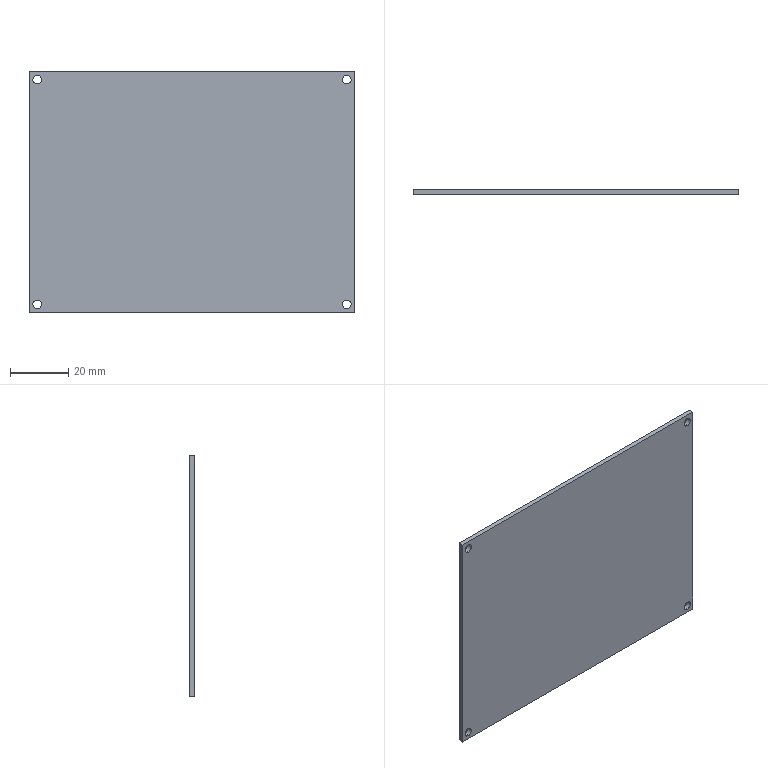Part | SolidWorks | features Extrusion 1 | 1 solid | 14 faces | box 111.5 x 1.75 x 82.6 mm | volume 16068 mm3 | cylinder 8 | plane 6 | commonest cylinder face diameters 3 x8
STEP:
#1=CARTESIAN_POINT('',(-53.,1.75,37.));
#2=VERTEX_POINT('',#1);
#3=CARTESIAN_POINT('',(-53.,1.75,40.));
#4=VERTEX_POINT('',#3);
#5=CARTESIAN_POINT('',(-53.,1.75,38.5));
#6=DIRECTION('',(0.,1.,0.));
#7=DIRECTION('',(0.,0.,-1.));
#8=AXIS2_PLACEMENT_3D('',#5,#6,#7);
#9=CIRCLE('',#8,1.5);
#10=EDGE_CURVE('',#2,#4,#9,.T.);
#11=ORIENTED_EDGE('',*,*,#10,.T.);
#12=CARTESIAN_POINT('',(-53.,0.,40.));
#13=VERTEX_POINT('',#12);
#14=CARTESIAN_POINT('',(-53.,1.75,40.));
#15=DIRECTION('',(0.,-1.,0.));
#16=VECTOR('',#15,1000.);
#17=LINE('',#14,#16);
#18=EDGE_CURVE('',#4,#13,#17,.T.);
#19=ORIENTED_EDGE('',*,*,#18,.T.);
#20=CARTESIAN_POINT('',(-53.,0.,37.));
#21=VERTEX_POINT('',#20);
#22=CARTESIAN_POINT('',(-53.,0.,38.5));
#23=DIRECTION('',(0.,1.,0.));
#24=DIRECTION('',(0.,0.,-1.));
#25=AXIS2_PLACEMENT_3D('',#22,#23,#24);
#26=CIRCLE('',#25,1.5);
#27=EDGE_CURVE('',#21,#13,#26,.T.);
#28=ORIENTED_EDGE('',*,*,#27,.F.);
#29=CARTESIAN_POINT('',(-53.,1.75,37.));
#30=DIRECTION('',(0.,-1.,0.));
#31=VECTOR('',#30,1000.);
#32=LINE('',#29,#31);
#33=EDGE_CURVE('',#2,#21,#32,.T.);
#34=ORIENTED_EDGE('',*,*,#33,.F.);
#35=EDGE_LOOP('',(#11,#19,#28,#34));
#36=FACE_OUTER_BOUND('',#35,.T.);
#37=CARTESIAN_POINT('',(-53.,1.75,38.5));
#38=DIRECTION('',(0.,-1.,0.));
#39=DIRECTION('',(0.,0.,-1.));
#40=AXIS2_PLACEMENT_3D('',#37,#38,#39);
#41=CYLINDRICAL_SURFACE('',#40,1.5);
#42=ADVANCED_FACE('',(#36),#41,.F.);
#43=CARTESIAN_POINT('',(53.,1.75,37.));
#44=VERTEX_POINT('',#43);
#45=CARTESIAN_POINT('',(53.,1.75,40.));
#46=VERTEX_POINT('',#45);
#47=CARTESIAN_POINT('',(53.,1.75,38.5));
#48=DIRECTION('',(0.,1.,0.));
#49=DIRECTION('',(0.,0.,1.));
#50=AXIS2_PLACEMENT_3D('',#47,#48,#49);
#51=CIRCLE('',#50,1.5);
#52=EDGE_CURVE('',#44,#46,#51,.T.);
#53=ORIENTED_EDGE('',*,*,#52,.T.);
#54=CARTESIAN_POINT('',(53.,0.,40.));
#55=VERTEX_POINT('',#54);
#56=CARTESIAN_POINT('',(53.,1.75,40.));
#57=DIRECTION('',(0.,-1.,0.));
#58=VECTOR('',#57,1000.);
#59=LINE('',#56,#58);
#60=EDGE_CURVE('',#46,#55,#59,.T.);
#61=ORIENTED_EDGE('',*,*,#60,.T.);
#62=CARTESIAN_POINT('',(53.,0.,37.));
#63=VERTEX_POINT('',#62);
#64=CARTESIAN_POINT('',(53.,0.,38.5));
#65=DIRECTION('',(0.,1.,0.));
#66=DIRECTION('',(0.,0.,1.));
#67=AXIS2_PLACEMENT_3D('',#64,#65,#66);
#68=CIRCLE('',#67,1.5);
#69=EDGE_CURVE('',#63,#55,#68,.T.);
#70=ORIENTED_EDGE('',*,*,#69,.F.);
#71=CARTESIAN_POINT('',(53.,1.75,37.));
#72=DIRECTION('',(0.,-1.,0.));
#73=VECTOR('',#72,1000.);
#74=LINE('',#71,#73);
#75=EDGE_CURVE('',#44,#63,#74,.T.);
#76=ORIENTED_EDGE('',*,*,#75,.F.);
#77=EDGE_LOOP('',(#53,#61,#70,#76));
#78=FACE_OUTER_BOUND('',#77,.T.);
#79=CARTESIAN_POINT('',(53.,1.75,38.5));
#80=DIRECTION('',(0.,-1.,0.));
#81=DIRECTION('',(0.,0.,-1.));
#82=AXIS2_PLACEMENT_3D('',#79,#80,#81);
#83=CYLINDRICAL_SURFACE('',#82,1.5);
#84=ADVANCED_FACE('',(#78),#83,.F.);
#85=CARTESIAN_POINT('',(53.,1.75,-40.));
#86=VERTEX_POINT('',#85);
#87=CARTESIAN_POINT('',(53.,1.75,-37.));
#88=VERTEX_POINT('',#87);
#89=CARTESIAN_POINT('',(53.,1.75,-38.5));
#90=DIRECTION('',(0.,1.,0.));
#91=DIRECTION('',(0.,0.,-1.));
#92=AXIS2_PLACEMENT_3D('',#89,#90,#91);
#93=CIRCLE('',#92,1.5);
#94=EDGE_CURVE('',#86,#88,#93,.T.);
#95=ORIENTED_EDGE('',*,*,#94,.T.);
#96=CARTESIAN_POINT('',(53.,0.,-37.));
#97=VERTEX_POINT('',#96);
#98=CARTESIAN_POINT('',(53.,1.75,-37.));
#99=DIRECTION('',(0.,-1.,0.));
#100=VECTOR('',#99,1000.);
#101=LINE('',#98,#100);
#102=EDGE_CURVE('',#88,#97,#101,.T.);
#103=ORIENTED_EDGE('',*,*,#102,.T.);
#104=CARTESIAN_POINT('',(53.,0.,-40.));
#105=VERTEX_POINT('',#104);
#106=CARTESIAN_POINT('',(53.,0.,-38.5));
#107=DIRECTION('',(0.,1.,0.));
#108=DIRECTION('',(0.,0.,-1.));
#109=AXIS2_PLACEMENT_3D('',#106,#107,#108);
#110=CIRCLE('',#109,1.5);
#111=EDGE_CURVE('',#105,#97,#110,.T.);
#112=ORIENTED_EDGE('',*,*,#111,.F.);
#113=CARTESIAN_POINT('',(53.,1.75,-40.));
#114=DIRECTION('',(0.,-1.,0.));
#115=VECTOR('',#114,1000.);
#116=LINE('',#113,#115);
#117=EDGE_CURVE('',#86,#105,#116,.T.);
#118=ORIENTED_EDGE('',*,*,#117,.F.);
#119=EDGE_LOOP('',(#95,#103,#112,#118));
#120=FACE_OUTER_BOUND('',#119,.T.);
#121=CARTESIAN_POINT('',(53.,1.75,-38.5));
#122=DIRECTION('',(0.,-1.,0.));
#123=DIRECTION('',(0.,0.,-1.));
#124=AXIS2_PLACEMENT_3D('',#121,#122,#123);
#125=CYLINDRICAL_SURFACE('',#124,1.5);
#126=ADVANCED_FACE('',(#120),#125,.F.);
#127=CARTESIAN_POINT('',(-53.,1.75,-40.));
#128=VERTEX_POINT('',#127);
#129=CARTESIAN_POINT('',(-53.,1.75,-37.));
#130=VERTEX_POINT('',#129);
#131=CARTESIAN_POINT('',(-53.,1.75,-38.5));
#132=DIRECTION('',(0.,1.,0.));
#133=DIRECTION('',(0.,0.,1.));
#134=AXIS2_PLACEMENT_3D('',#131,#132,#133);
#135=CIRCLE('',#134,1.5);
#136=EDGE_CURVE('',#128,#130,#135,.T.);
#137=ORIENTED_EDGE('',*,*,#136,.T.);
#138=CARTESIAN_POINT('',(-53.,0.,-37.));
#139=VERTEX_POINT('',#138);
#140=CARTESIAN_POINT('',(-53.,1.75,-37.));
#141=DIRECTION('',(0.,-1.,0.));
#142=VECTOR('',#141,1000.);
#143=LINE('',#140,#142);
#144=EDGE_CURVE('',#130,#139,#143,.T.);
#145=ORIENTED_EDGE('',*,*,#144,.T.);
#146=CARTESIAN_POINT('',(-53.,0.,-40.));
#147=VERTEX_POINT('',#146);
#148=CARTESIAN_POINT('',(-53.,0.,-38.5));
#149=DIRECTION('',(0.,1.,0.));
#150=DIRECTION('',(0.,0.,1.));
#151=AXIS2_PLACEMENT_3D('',#148,#149,#150);
#152=CIRCLE('',#151,1.5);
#153=EDGE_CURVE('',#147,#139,#152,.T.);
#154=ORIENTED_EDGE('',*,*,#153,.F.);
#155=CARTESIAN_POINT('',(-53.,1.75,-40.));
#156=DIRECTION('',(0.,-1.,0.));
#157=VECTOR('',#156,1000.);
#158=LINE('',#155,#157);
#159=EDGE_CURVE('',#128,#147,#158,.T.);
#160=ORIENTED_EDGE('',*,*,#159,.F.);
#161=EDGE_LOOP('',(#137,#145,#154,#160));
#162=FACE_OUTER_BOUND('',#161,.T.);
#163=CARTESIAN_POINT('',(-53.,1.75,-38.5));
#164=DIRECTION('',(0.,-1.,0.));
#165=DIRECTION('',(0.,0.,-1.));
#166=AXIS2_PLACEMENT_3D('',#163,#164,#165);
#167=CYLINDRICAL_SURFACE('',#166,1.5);
#168=ADVANCED_FACE('',(#162),#167,.F.);
#169=ORIENTED_EDGE('',*,*,#52,.F.);
#170=CARTESIAN_POINT('',(53.,1.75,38.5));
#171=DIRECTION('',(0.,1.,0.));
#172=DIRECTION('',(0.,0.,1.));
#173=AXIS2_PLACEMENT_3D('',#170,#171,#172);
#174=CIRCLE('',#173,1.5);
#175=EDGE_CURVE('',#46,#44,#174,.T.);
#176=ORIENTED_EDGE('',*,*,#175,.F.);
#177=EDGE_LOOP('',(#169,#176));
#178=FACE_BOUND('',#177,.T.);
#179=ORIENTED_EDGE('',*,*,#136,.F.);
#180=CARTESIAN_POINT('',(-53.,1.75,-38.5));
#181=DIRECTION('',(0.,1.,0.));
#182=DIRECTION('',(0.,0.,1.));
#183=AXIS2_PLACEMENT_3D('',#180,#181,#182);
#184=CIRCLE('',#183,1.5);
#185=EDGE_CURVE('',#130,#128,#184,.T.);
#186=ORIENTED_EDGE('',*,*,#185,.F.);
#187=EDGE_LOOP('',(#179,#186));
#188=FACE_BOUND('',#187,.T.);
#189=CARTESIAN_POINT('',(55.75,1.75,41.3));
#190=VERTEX_POINT('',#189);
#191=CARTESIAN_POINT('',(55.75,1.75,-41.3));
#192=VERTEX_POINT('',#191);
#193=CARTESIAN_POINT('',(55.75,1.75,41.3));
#194=DIRECTION('',(0.,0.,-1.));
#195=VECTOR('',#194,1000.);
#196=LINE('',#193,#195);
#197=EDGE_CURVE('',#190,#192,#196,.T.);
#198=ORIENTED_EDGE('',*,*,#197,.T.);
#199=CARTESIAN_POINT('',(-55.75,1.75,-41.3));
#200=VERTEX_POINT('',#199);
#201=CARTESIAN_POINT('',(-55.75,1.75,-41.3));
#202=DIRECTION('',(-1.,0.,0.));
#203=VECTOR('',#202,1000.);
#204=LINE('',#201,#203);
#205=EDGE_CURVE('',#192,#200,#204,.T.);
#206=ORIENTED_EDGE('',*,*,#205,.T.);
#207=CARTESIAN_POINT('',(-55.75,1.75,41.3));
#208=VERTEX_POINT('',#207);
#209=CARTESIAN_POINT('',(-55.75,1.75,41.3));
#210=DIRECTION('',(0.,0.,1.));
#211=VECTOR('',#210,1000.);
#212=LINE('',#209,#211);
#213=EDGE_CURVE('',#200,#208,#212,.T.);
#214=ORIENTED_EDGE('',*,*,#213,.T.);
#215=CARTESIAN_POINT('',(-55.75,1.75,41.3));
#216=DIRECTION('',(1.,0.,0.));
#217=VECTOR('',#216,1000.);
#218=LINE('',#215,#217);
#219=EDGE_CURVE('',#208,#190,#218,.T.);
#220=ORIENTED_EDGE('',*,*,#219,.T.);
#221=EDGE_LOOP('',(#198,#206,#214,#220));
#222=FACE_OUTER_BOUND('',#221,.T.);
#223=ORIENTED_EDGE('',*,*,#94,.F.);
#224=CARTESIAN_POINT('',(53.,1.75,-38.5));
#225=DIRECTION('',(0.,1.,0.));
#226=DIRECTION('',(0.,0.,-1.));
#227=AXIS2_PLACEMENT_3D('',#224,#225,#226);
#228=CIRCLE('',#227,1.5);
#229=EDGE_CURVE('',#88,#86,#228,.T.);
#230=ORIENTED_EDGE('',*,*,#229,.F.);
#231=EDGE_LOOP('',(#223,#230));
#232=FACE_BOUND('',#231,.T.);
#233=ORIENTED_EDGE('',*,*,#10,.F.);
#234=CARTESIAN_POINT('',(-53.,1.75,38.5));
#235=DIRECTION('',(0.,1.,0.));
#236=DIRECTION('',(0.,0.,-1.));
#237=AXIS2_PLACEMENT_3D('',#234,#235,#236);
#238=CIRCLE('',#237,1.5);
#239=EDGE_CURVE('',#4,#2,#238,.T.);
#240=ORIENTED_EDGE('',*,*,#239,.F.);
#241=EDGE_LOOP('',(#233,#240));
#242=FACE_BOUND('',#241,.T.);
#243=CARTESIAN_POINT('',(0.,1.75,0.));
#244=DIRECTION('',(0.,-1.,0.));
#245=DIRECTION('',(0.,0.,-1.));
#246=AXIS2_PLACEMENT_3D('',#243,#244,#245);
#247=PLANE('',#246);
#248=ADVANCED_FACE('',(#178,#188,#222,#232,#242),#247,.F.);
#249=ORIENTED_EDGE('',*,*,#69,.T.);
#250=CARTESIAN_POINT('',(53.,0.,38.5));
#251=DIRECTION('',(0.,1.,0.));
#252=DIRECTION('',(0.,0.,1.));
#253=AXIS2_PLACEMENT_3D('',#250,#251,#252);
#254=CIRCLE('',#253,1.5);
#255=EDGE_CURVE('',#55,#63,#254,.T.);
#256=ORIENTED_EDGE('',*,*,#255,.T.);
#257=EDGE_LOOP('',(#249,#256));
#258=FACE_BOUND('',#257,.T.);
#259=ORIENTED_EDGE('',*,*,#153,.T.);
#260=CARTESIAN_POINT('',(-53.,0.,-38.5));
#261=DIRECTION('',(0.,1.,0.));
#262=DIRECTION('',(0.,0.,1.));
#263=AXIS2_PLACEMENT_3D('',#260,#261,#262);
#264=CIRCLE('',#263,1.5);
#265=EDGE_CURVE('',#139,#147,#264,.T.);
#266=ORIENTED_EDGE('',*,*,#265,.T.);
#267=EDGE_LOOP('',(#259,#266));
#268=FACE_BOUND('',#267,.T.);
#269=CARTESIAN_POINT('',(55.75,0.,41.3));
#270=VERTEX_POINT('',#269);
#271=CARTESIAN_POINT('',(55.75,0.,-41.3));
#272=VERTEX_POINT('',#271);
#273=CARTESIAN_POINT('',(55.75,0.,41.3));
#274=DIRECTION('',(0.,0.,-1.));
#275=VECTOR('',#274,1000.);
#276=LINE('',#273,#275);
#277=EDGE_CURVE('',#270,#272,#276,.T.);
#278=ORIENTED_EDGE('',*,*,#277,.F.);
#279=CARTESIAN_POINT('',(-55.75,0.,41.3));
#280=VERTEX_POINT('',#279);
#281=CARTESIAN_POINT('',(-55.75,0.,41.3));
#282=DIRECTION('',(1.,0.,0.));
#283=VECTOR('',#282,1000.);
#284=LINE('',#281,#283);
#285=EDGE_CURVE('',#280,#270,#284,.T.);
#286=ORIENTED_EDGE('',*,*,#285,.F.);
#287=CARTESIAN_POINT('',(-55.75,0.,-41.3));
#288=VERTEX_POINT('',#287);
#289=CARTESIAN_POINT('',(-55.75,0.,41.3));
#290=DIRECTION('',(0.,0.,1.));
#291=VECTOR('',#290,1000.);
#292=LINE('',#289,#291);
#293=EDGE_CURVE('',#288,#280,#292,.T.);
#294=ORIENTED_EDGE('',*,*,#293,.F.);
#295=CARTESIAN_POINT('',(-55.75,0.,-41.3));
#296=DIRECTION('',(-1.,0.,0.));
#297=VECTOR('',#296,1000.);
#298=LINE('',#295,#297);
#299=EDGE_CURVE('',#272,#288,#298,.T.);
#300=ORIENTED_EDGE('',*,*,#299,.F.);
#301=EDGE_LOOP('',(#278,#286,#294,#300));
#302=FACE_OUTER_BOUND('',#301,.T.);
#303=ORIENTED_EDGE('',*,*,#111,.T.);
#304=CARTESIAN_POINT('',(53.,0.,-38.5));
#305=DIRECTION('',(0.,1.,0.));
#306=DIRECTION('',(0.,0.,-1.));
#307=AXIS2_PLACEMENT_3D('',#304,#305,#306);
#308=CIRCLE('',#307,1.5);
#309=EDGE_CURVE('',#97,#105,#308,.T.);
#310=ORIENTED_EDGE('',*,*,#309,.T.);
#311=EDGE_LOOP('',(#303,#310));
#312=FACE_BOUND('',#311,.T.);
#313=ORIENTED_EDGE('',*,*,#27,.T.);
#314=CARTESIAN_POINT('',(-53.,0.,38.5));
#315=DIRECTION('',(0.,1.,0.));
#316=DIRECTION('',(0.,0.,-1.));
#317=AXIS2_PLACEMENT_3D('',#314,#315,#316);
#318=CIRCLE('',#317,1.5);
#319=EDGE_CURVE('',#13,#21,#318,.T.);
#320=ORIENTED_EDGE('',*,*,#319,.T.);
#321=EDGE_LOOP('',(#313,#320));
#322=FACE_BOUND('',#321,.T.);
#323=CARTESIAN_POINT('',(0.,0.,0.));
#324=DIRECTION('',(0.,-1.,0.));
#325=DIRECTION('',(0.,0.,-1.));
#326=AXIS2_PLACEMENT_3D('',#323,#324,#325);
#327=PLANE('',#326);
#328=ADVANCED_FACE('',(#258,#268,#302,#312,#322),#327,.T.);
#329=ORIENTED_EDGE('',*,*,#277,.T.);
#330=CARTESIAN_POINT('',(55.75,1.75,-41.3));
#331=DIRECTION('',(0.,-1.,0.));
#332=VECTOR('',#331,1000.);
#333=LINE('',#330,#332);
#334=EDGE_CURVE('',#192,#272,#333,.T.);
#335=ORIENTED_EDGE('',*,*,#334,.F.);
#336=ORIENTED_EDGE('',*,*,#197,.F.);
#337=CARTESIAN_POINT('',(55.75,1.75,41.3));
#338=DIRECTION('',(0.,-1.,0.));
#339=VECTOR('',#338,1000.);
#340=LINE('',#337,#339);
#341=EDGE_CURVE('',#190,#270,#340,.T.);
#342=ORIENTED_EDGE('',*,*,#341,.T.);
#343=EDGE_LOOP('',(#329,#335,#336,#342));
#344=FACE_OUTER_BOUND('',#343,.T.);
#345=CARTESIAN_POINT('',(55.75,1.75,41.3));
#346=DIRECTION('',(-1.,0.,0.));
#347=DIRECTION('',(0.,0.,1.));
#348=AXIS2_PLACEMENT_3D('',#345,#346,#347);
#349=PLANE('',#348);
#350=ADVANCED_FACE('',(#344),#349,.F.);
#351=ORIENTED_EDGE('',*,*,#299,.T.);
#352=CARTESIAN_POINT('',(-55.75,1.75,-41.3));
#353=DIRECTION('',(0.,-1.,0.));
#354=VECTOR('',#353,1000.);
#355=LINE('',#352,#354);
#356=EDGE_CURVE('',#200,#288,#355,.T.);
#357=ORIENTED_EDGE('',*,*,#356,.F.);
#358=ORIENTED_EDGE('',*,*,#205,.F.);
#359=ORIENTED_EDGE('',*,*,#334,.T.);
#360=EDGE_LOOP('',(#351,#357,#358,#359));
#361=FACE_OUTER_BOUND('',#360,.T.);
#362=CARTESIAN_POINT('',(-55.75,1.75,-41.3));
#363=DIRECTION('',(0.,0.,1.));
#364=DIRECTION('',(1.,0.,0.));
#365=AXIS2_PLACEMENT_3D('',#362,#363,#364);
#366=PLANE('',#365);
#367=ADVANCED_FACE('',(#361),#366,.F.);
#368=ORIENTED_EDGE('',*,*,#293,.T.);
#369=CARTESIAN_POINT('',(-55.75,1.75,41.3));
#370=DIRECTION('',(0.,-1.,0.));
#371=VECTOR('',#370,1000.);
#372=LINE('',#369,#371);
#373=EDGE_CURVE('',#208,#280,#372,.T.);
#374=ORIENTED_EDGE('',*,*,#373,.F.);
#375=ORIENTED_EDGE('',*,*,#213,.F.);
#376=ORIENTED_EDGE('',*,*,#356,.T.);
#377=EDGE_LOOP('',(#368,#374,#375,#376));
#378=FACE_OUTER_BOUND('',#377,.T.);
#379=CARTESIAN_POINT('',(-55.75,1.75,41.3));
#380=DIRECTION('',(1.,0.,0.));
#381=DIRECTION('',(0.,0.,-1.));
#382=AXIS2_PLACEMENT_3D('',#379,#380,#381);
#383=PLANE('',#382);
#384=ADVANCED_FACE('',(#378),#383,.F.);
#385=ORIENTED_EDGE('',*,*,#285,.T.);
#386=ORIENTED_EDGE('',*,*,#341,.F.);
#387=ORIENTED_EDGE('',*,*,#219,.F.);
#388=ORIENTED_EDGE('',*,*,#373,.T.);
#389=EDGE_LOOP('',(#385,#386,#387,#388));
#390=FACE_OUTER_BOUND('',#389,.T.);
#391=CARTESIAN_POINT('',(-55.75,1.75,41.3));
#392=DIRECTION('',(0.,0.,-1.));
#393=DIRECTION('',(-1.,0.,0.));
#394=AXIS2_PLACEMENT_3D('',#391,#392,#393);
#395=PLANE('',#394);
#396=ADVANCED_FACE('',(#390),#395,.F.);
#397=ORIENTED_EDGE('',*,*,#144,.F.);
#398=ORIENTED_EDGE('',*,*,#185,.T.);
#399=ORIENTED_EDGE('',*,*,#159,.T.);
#400=ORIENTED_EDGE('',*,*,#265,.F.);
#401=EDGE_LOOP('',(#397,#398,#399,#400));
#402=FACE_OUTER_BOUND('',#401,.T.);
#403=CARTESIAN_POINT('',(-53.,1.75,-38.5));
#404=DIRECTION('',(0.,-1.,0.));
#405=DIRECTION('',(0.,0.,-1.));
#406=AXIS2_PLACEMENT_3D('',#403,#404,#405);
#407=CYLINDRICAL_SURFACE('',#406,1.5);
#408=ADVANCED_FACE('',(#402),#407,.F.);
#409=ORIENTED_EDGE('',*,*,#102,.F.);
#410=ORIENTED_EDGE('',*,*,#229,.T.);
#411=ORIENTED_EDGE('',*,*,#117,.T.);
#412=ORIENTED_EDGE('',*,*,#309,.F.);
#413=EDGE_LOOP('',(#409,#410,#411,#412));
#414=FACE_OUTER_BOUND('',#413,.T.);
#415=CARTESIAN_POINT('',(53.,1.75,-38.5));
#416=DIRECTION('',(0.,-1.,0.));
#417=DIRECTION('',(0.,0.,-1.));
#418=AXIS2_PLACEMENT_3D('',#415,#416,#417);
#419=CYLINDRICAL_SURFACE('',#418,1.5);
#420=ADVANCED_FACE('',(#414),#419,.F.);
#421=ORIENTED_EDGE('',*,*,#60,.F.);
#422=ORIENTED_EDGE('',*,*,#175,.T.);
#423=ORIENTED_EDGE('',*,*,#75,.T.);
#424=ORIENTED_EDGE('',*,*,#255,.F.);
#425=EDGE_LOOP('',(#421,#422,#423,#424));
#426=FACE_OUTER_BOUND('',#425,.T.);
#427=CARTESIAN_POINT('',(53.,1.75,38.5));
#428=DIRECTION('',(0.,-1.,0.));
#429=DIRECTION('',(0.,0.,-1.));
#430=AXIS2_PLACEMENT_3D('',#427,#428,#429);
#431=CYLINDRICAL_SURFACE('',#430,1.5);
#432=ADVANCED_FACE('',(#426),#431,.F.);
#433=ORIENTED_EDGE('',*,*,#18,.F.);
#434=ORIENTED_EDGE('',*,*,#239,.T.);
#435=ORIENTED_EDGE('',*,*,#33,.T.);
#436=ORIENTED_EDGE('',*,*,#319,.F.);
#437=EDGE_LOOP('',(#433,#434,#435,#436));
#438=FACE_OUTER_BOUND('',#437,.T.);
#439=CARTESIAN_POINT('',(-53.,1.75,38.5));
#440=DIRECTION('',(0.,-1.,0.));
#441=DIRECTION('',(0.,0.,-1.));
#442=AXIS2_PLACEMENT_3D('',#439,#440,#441);
#443=CYLINDRICAL_SURFACE('',#442,1.5);
#444=ADVANCED_FACE('',(#438),#443,.F.);
#445=CLOSED_SHELL('',(#42,#84,#126,#168,#248,#328,#350,#367,#384,#396,#408,#420,#432,#444));
#446=MANIFOLD_SOLID_BREP('',#445);
#447=CARTESIAN_POINT('',(0.,0.,0.));
#448=DIRECTION('',(0.,0.,1.));
#449=DIRECTION('',(1.,0.,0.));
#450=AXIS2_PLACEMENT_3D('',#447,#448,#449);
#451=(LENGTH_UNIT()NAMED_UNIT(*)SI_UNIT(.MILLI.,.METRE.));
#452=UNCERTAINTY_MEASURE_WITH_UNIT(LENGTH_MEASURE(0.00001),#451,'','');
#453=(NAMED_UNIT(*)PLANE_ANGLE_UNIT()SI_UNIT($,.RADIAN.));
#454=(NAMED_UNIT(*)SI_UNIT($,.STERADIAN.)SOLID_ANGLE_UNIT());
#455=(GEOMETRIC_REPRESENTATION_CONTEXT(3)GLOBAL_UNCERTAINTY_ASSIGNED_CONTEXT((#452))GLOBAL_UNIT_ASSIGNED_CONTEXT((#451,#453,#454))REPRESENTATION_CONTEXT('',''));
#456=ADVANCED_BREP_SHAPE_REPRESENTATION('',(#446,#450),#455);